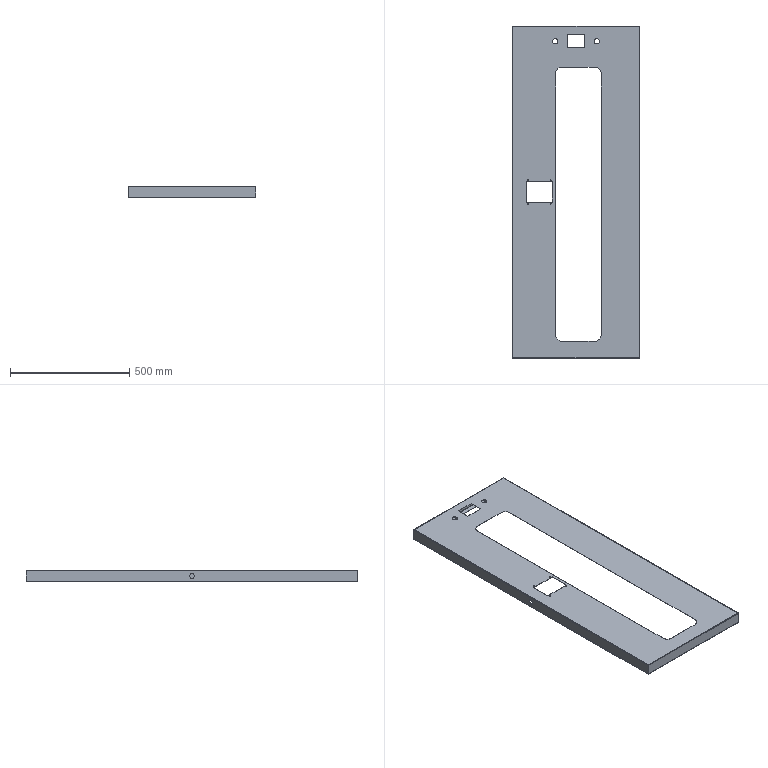Part | SolidWorks | features ICE 3, EdgeFlange 2, CornerFeat 1, Cut 1, FlatPattern 1, SMBaseFlange 1, SheetMetal 1 | 1 solid | 102 faces | box 536 x 1392 x 48.5 mm | volume 914346 mm3 | plane 51 | cylinder 35 | spline 16 | commonest cylinder face diameters 1.473 x8 3.873 x8 5 x8 22 x5 50 x4 20 x2